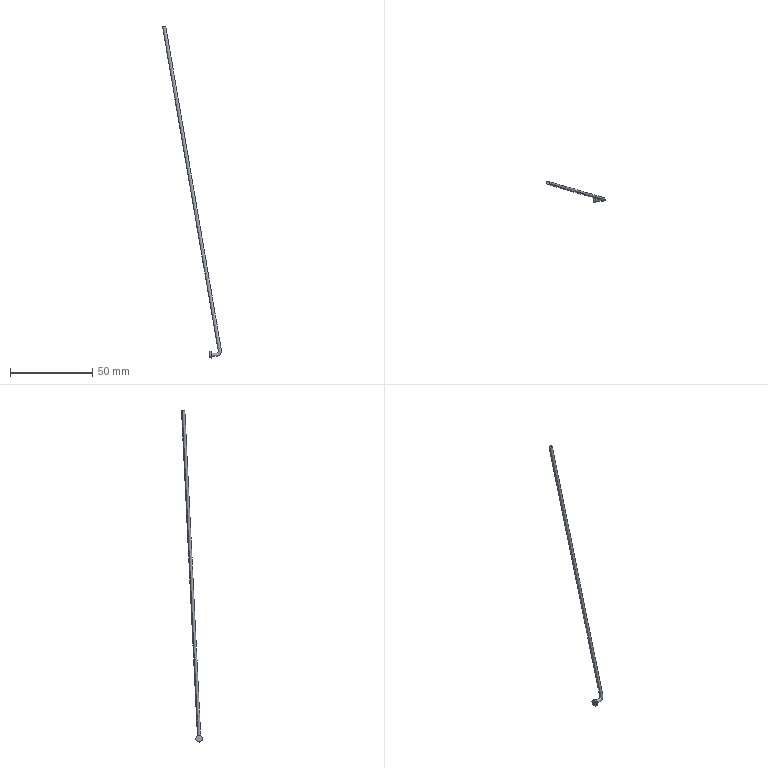Part | STEP file | BREP_79 | 1 solid | 7 faces | box 35.925 x 12.735 x 202.012 mm | volume 668.221 mm3 | plane 3 | spline 2 | cylinder 2 | commonest cylinder face diameters 4 x2